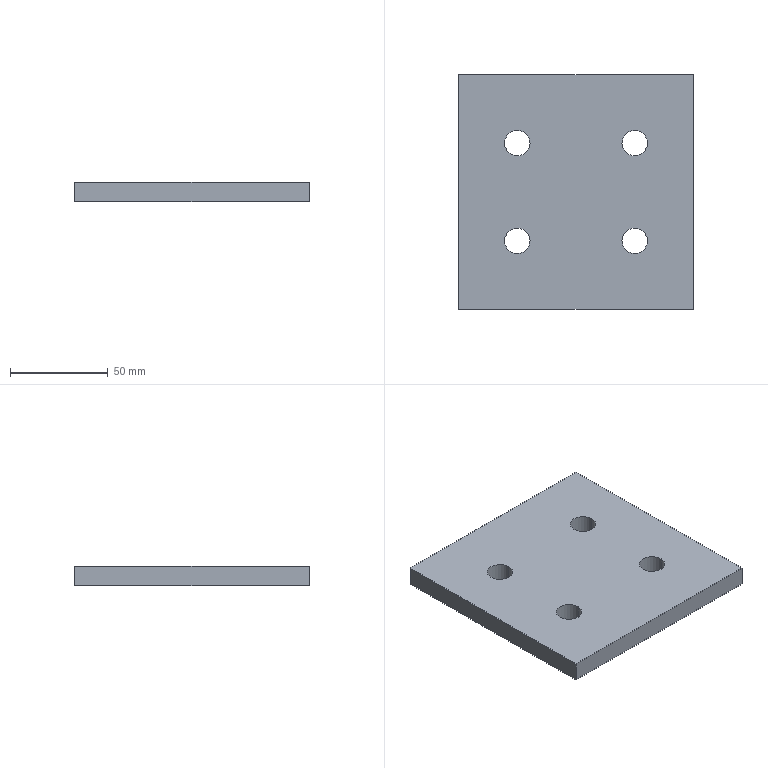Part | SolidWorks | features Extrusion 1 | 1 solid | 14 faces | box 120 x 120 x 10 mm | volume 138691 mm3 | cylinder 8 | plane 6 | commonest cylinder face diameters 13 x8
STEP:
#1=CARTESIAN_POINT('',(23.5,35.,10.));
#2=VERTEX_POINT('',#1);
#3=CARTESIAN_POINT('',(36.5,35.,10.));
#4=VERTEX_POINT('',#3);
#5=CARTESIAN_POINT('',(30.,35.,10.));
#6=DIRECTION('',(0.,0.,1.));
#7=DIRECTION('',(1.,0.,0.));
#8=AXIS2_PLACEMENT_3D('',#5,#6,#7);
#9=CIRCLE('',#8,6.5);
#10=EDGE_CURVE('',#2,#4,#9,.T.);
#11=ORIENTED_EDGE('',*,*,#10,.T.);
#12=CARTESIAN_POINT('',(36.5,35.,0.));
#13=VERTEX_POINT('',#12);
#14=CARTESIAN_POINT('',(36.5,35.,10.));
#15=DIRECTION('',(0.,0.,-1.));
#16=VECTOR('',#15,1000.);
#17=LINE('',#14,#16);
#18=EDGE_CURVE('',#4,#13,#17,.T.);
#19=ORIENTED_EDGE('',*,*,#18,.T.);
#20=CARTESIAN_POINT('',(23.5,35.,0.));
#21=VERTEX_POINT('',#20);
#22=CARTESIAN_POINT('',(30.,35.,0.));
#23=DIRECTION('',(0.,0.,1.));
#24=DIRECTION('',(1.,0.,0.));
#25=AXIS2_PLACEMENT_3D('',#22,#23,#24);
#26=CIRCLE('',#25,6.5);
#27=EDGE_CURVE('',#21,#13,#26,.T.);
#28=ORIENTED_EDGE('',*,*,#27,.F.);
#29=CARTESIAN_POINT('',(23.5,35.,10.));
#30=DIRECTION('',(0.,0.,-1.));
#31=VECTOR('',#30,1000.);
#32=LINE('',#29,#31);
#33=EDGE_CURVE('',#2,#21,#32,.T.);
#34=ORIENTED_EDGE('',*,*,#33,.F.);
#35=EDGE_LOOP('',(#11,#19,#28,#34));
#36=FACE_OUTER_BOUND('',#35,.T.);
#37=CARTESIAN_POINT('',(30.,35.,10.));
#38=DIRECTION('',(0.,0.,-1.));
#39=DIRECTION('',(-1.,0.,0.));
#40=AXIS2_PLACEMENT_3D('',#37,#38,#39);
#41=CYLINDRICAL_SURFACE('',#40,6.5);
#42=ADVANCED_FACE('',(#36),#41,.F.);
#43=CARTESIAN_POINT('',(23.5,85.,10.));
#44=VERTEX_POINT('',#43);
#45=CARTESIAN_POINT('',(36.5,85.,10.));
#46=VERTEX_POINT('',#45);
#47=CARTESIAN_POINT('',(30.,85.,10.));
#48=DIRECTION('',(0.,0.,1.));
#49=DIRECTION('',(1.,0.,0.));
#50=AXIS2_PLACEMENT_3D('',#47,#48,#49);
#51=CIRCLE('',#50,6.5);
#52=EDGE_CURVE('',#44,#46,#51,.T.);
#53=ORIENTED_EDGE('',*,*,#52,.T.);
#54=CARTESIAN_POINT('',(36.5,85.,0.));
#55=VERTEX_POINT('',#54);
#56=CARTESIAN_POINT('',(36.5,85.,10.));
#57=DIRECTION('',(0.,0.,-1.));
#58=VECTOR('',#57,1000.);
#59=LINE('',#56,#58);
#60=EDGE_CURVE('',#46,#55,#59,.T.);
#61=ORIENTED_EDGE('',*,*,#60,.T.);
#62=CARTESIAN_POINT('',(23.5,85.,0.));
#63=VERTEX_POINT('',#62);
#64=CARTESIAN_POINT('',(30.,85.,0.));
#65=DIRECTION('',(0.,0.,1.));
#66=DIRECTION('',(1.,0.,0.));
#67=AXIS2_PLACEMENT_3D('',#64,#65,#66);
#68=CIRCLE('',#67,6.5);
#69=EDGE_CURVE('',#63,#55,#68,.T.);
#70=ORIENTED_EDGE('',*,*,#69,.F.);
#71=CARTESIAN_POINT('',(23.5,85.,10.));
#72=DIRECTION('',(0.,0.,-1.));
#73=VECTOR('',#72,1000.);
#74=LINE('',#71,#73);
#75=EDGE_CURVE('',#44,#63,#74,.T.);
#76=ORIENTED_EDGE('',*,*,#75,.F.);
#77=EDGE_LOOP('',(#53,#61,#70,#76));
#78=FACE_OUTER_BOUND('',#77,.T.);
#79=CARTESIAN_POINT('',(30.,85.,10.));
#80=DIRECTION('',(0.,0.,-1.));
#81=DIRECTION('',(-1.,0.,0.));
#82=AXIS2_PLACEMENT_3D('',#79,#80,#81);
#83=CYLINDRICAL_SURFACE('',#82,6.5);
#84=ADVANCED_FACE('',(#78),#83,.F.);
#85=CARTESIAN_POINT('',(83.5,85.,10.));
#86=VERTEX_POINT('',#85);
#87=CARTESIAN_POINT('',(96.5,85.,10.));
#88=VERTEX_POINT('',#87);
#89=CARTESIAN_POINT('',(90.,85.,10.));
#90=DIRECTION('',(0.,0.,1.));
#91=DIRECTION('',(1.,0.,0.));
#92=AXIS2_PLACEMENT_3D('',#89,#90,#91);
#93=CIRCLE('',#92,6.5);
#94=EDGE_CURVE('',#86,#88,#93,.T.);
#95=ORIENTED_EDGE('',*,*,#94,.T.);
#96=CARTESIAN_POINT('',(96.5,85.,0.));
#97=VERTEX_POINT('',#96);
#98=CARTESIAN_POINT('',(96.5,85.,10.));
#99=DIRECTION('',(0.,0.,-1.));
#100=VECTOR('',#99,1000.);
#101=LINE('',#98,#100);
#102=EDGE_CURVE('',#88,#97,#101,.T.);
#103=ORIENTED_EDGE('',*,*,#102,.T.);
#104=CARTESIAN_POINT('',(83.5,85.,0.));
#105=VERTEX_POINT('',#104);
#106=CARTESIAN_POINT('',(90.,85.,0.));
#107=DIRECTION('',(0.,0.,1.));
#108=DIRECTION('',(1.,0.,0.));
#109=AXIS2_PLACEMENT_3D('',#106,#107,#108);
#110=CIRCLE('',#109,6.5);
#111=EDGE_CURVE('',#105,#97,#110,.T.);
#112=ORIENTED_EDGE('',*,*,#111,.F.);
#113=CARTESIAN_POINT('',(83.5,85.,10.));
#114=DIRECTION('',(0.,0.,-1.));
#115=VECTOR('',#114,1000.);
#116=LINE('',#113,#115);
#117=EDGE_CURVE('',#86,#105,#116,.T.);
#118=ORIENTED_EDGE('',*,*,#117,.F.);
#119=EDGE_LOOP('',(#95,#103,#112,#118));
#120=FACE_OUTER_BOUND('',#119,.T.);
#121=CARTESIAN_POINT('',(90.,85.,10.));
#122=DIRECTION('',(0.,0.,-1.));
#123=DIRECTION('',(-1.,0.,0.));
#124=AXIS2_PLACEMENT_3D('',#121,#122,#123);
#125=CYLINDRICAL_SURFACE('',#124,6.5);
#126=ADVANCED_FACE('',(#120),#125,.F.);
#127=CARTESIAN_POINT('',(83.5,35.,10.));
#128=VERTEX_POINT('',#127);
#129=CARTESIAN_POINT('',(96.5,35.,10.));
#130=VERTEX_POINT('',#129);
#131=CARTESIAN_POINT('',(90.,35.,10.));
#132=DIRECTION('',(0.,0.,1.));
#133=DIRECTION('',(1.,0.,0.));
#134=AXIS2_PLACEMENT_3D('',#131,#132,#133);
#135=CIRCLE('',#134,6.5);
#136=EDGE_CURVE('',#128,#130,#135,.T.);
#137=ORIENTED_EDGE('',*,*,#136,.T.);
#138=CARTESIAN_POINT('',(96.5,35.,0.));
#139=VERTEX_POINT('',#138);
#140=CARTESIAN_POINT('',(96.5,35.,10.));
#141=DIRECTION('',(0.,0.,-1.));
#142=VECTOR('',#141,1000.);
#143=LINE('',#140,#142);
#144=EDGE_CURVE('',#130,#139,#143,.T.);
#145=ORIENTED_EDGE('',*,*,#144,.T.);
#146=CARTESIAN_POINT('',(83.5,35.,0.));
#147=VERTEX_POINT('',#146);
#148=CARTESIAN_POINT('',(90.,35.,0.));
#149=DIRECTION('',(0.,0.,1.));
#150=DIRECTION('',(1.,0.,0.));
#151=AXIS2_PLACEMENT_3D('',#148,#149,#150);
#152=CIRCLE('',#151,6.5);
#153=EDGE_CURVE('',#147,#139,#152,.T.);
#154=ORIENTED_EDGE('',*,*,#153,.F.);
#155=CARTESIAN_POINT('',(83.5,35.,10.));
#156=DIRECTION('',(0.,0.,-1.));
#157=VECTOR('',#156,1000.);
#158=LINE('',#155,#157);
#159=EDGE_CURVE('',#128,#147,#158,.T.);
#160=ORIENTED_EDGE('',*,*,#159,.F.);
#161=EDGE_LOOP('',(#137,#145,#154,#160));
#162=FACE_OUTER_BOUND('',#161,.T.);
#163=CARTESIAN_POINT('',(90.,35.,10.));
#164=DIRECTION('',(0.,0.,-1.));
#165=DIRECTION('',(-1.,0.,0.));
#166=AXIS2_PLACEMENT_3D('',#163,#164,#165);
#167=CYLINDRICAL_SURFACE('',#166,6.5);
#168=ADVANCED_FACE('',(#162),#167,.F.);
#169=CARTESIAN_POINT('',(120.,0.,0.));
#170=VERTEX_POINT('',#169);
#171=CARTESIAN_POINT('',(0.,0.,0.));
#172=VERTEX_POINT('',#171);
#173=CARTESIAN_POINT('',(0.,0.,0.));
#174=DIRECTION('',(-1.,0.,0.));
#175=VECTOR('',#174,1000.);
#176=LINE('',#173,#175);
#177=EDGE_CURVE('',#170,#172,#176,.T.);
#178=ORIENTED_EDGE('',*,*,#177,.F.);
#179=CARTESIAN_POINT('',(120.,0.,10.));
#180=VERTEX_POINT('',#179);
#181=CARTESIAN_POINT('',(120.,0.,10.));
#182=DIRECTION('',(0.,0.,-1.));
#183=VECTOR('',#182,1000.);
#184=LINE('',#181,#183);
#185=EDGE_CURVE('',#180,#170,#184,.T.);
#186=ORIENTED_EDGE('',*,*,#185,.F.);
#187=CARTESIAN_POINT('',(0.,0.,10.));
#188=VERTEX_POINT('',#187);
#189=CARTESIAN_POINT('',(0.,0.,10.));
#190=DIRECTION('',(-1.,0.,0.));
#191=VECTOR('',#190,1000.);
#192=LINE('',#189,#191);
#193=EDGE_CURVE('',#180,#188,#192,.T.);
#194=ORIENTED_EDGE('',*,*,#193,.T.);
#195=CARTESIAN_POINT('',(0.,0.,10.));
#196=DIRECTION('',(0.,0.,-1.));
#197=VECTOR('',#196,1000.);
#198=LINE('',#195,#197);
#199=EDGE_CURVE('',#188,#172,#198,.T.);
#200=ORIENTED_EDGE('',*,*,#199,.T.);
#201=EDGE_LOOP('',(#178,#186,#194,#200));
#202=FACE_OUTER_BOUND('',#201,.T.);
#203=CARTESIAN_POINT('',(0.,0.,10.));
#204=DIRECTION('',(0.,-1.,0.));
#205=DIRECTION('',(0.,0.,-1.));
#206=AXIS2_PLACEMENT_3D('',#203,#204,#205);
#207=PLANE('',#206);
#208=ADVANCED_FACE('',(#202),#207,.T.);
#209=CARTESIAN_POINT('',(120.,120.,0.));
#210=VERTEX_POINT('',#209);
#211=CARTESIAN_POINT('',(120.,0.,0.));
#212=DIRECTION('',(0.,-1.,0.));
#213=VECTOR('',#212,1000.);
#214=LINE('',#211,#213);
#215=EDGE_CURVE('',#210,#170,#214,.T.);
#216=ORIENTED_EDGE('',*,*,#215,.F.);
#217=CARTESIAN_POINT('',(120.,120.,10.));
#218=VERTEX_POINT('',#217);
#219=CARTESIAN_POINT('',(120.,120.,10.));
#220=DIRECTION('',(0.,0.,-1.));
#221=VECTOR('',#220,1000.);
#222=LINE('',#219,#221);
#223=EDGE_CURVE('',#218,#210,#222,.T.);
#224=ORIENTED_EDGE('',*,*,#223,.F.);
#225=CARTESIAN_POINT('',(120.,0.,10.));
#226=DIRECTION('',(0.,-1.,0.));
#227=VECTOR('',#226,1000.);
#228=LINE('',#225,#227);
#229=EDGE_CURVE('',#218,#180,#228,.T.);
#230=ORIENTED_EDGE('',*,*,#229,.T.);
#231=ORIENTED_EDGE('',*,*,#185,.T.);
#232=EDGE_LOOP('',(#216,#224,#230,#231));
#233=FACE_OUTER_BOUND('',#232,.T.);
#234=CARTESIAN_POINT('',(120.,0.,10.));
#235=DIRECTION('',(1.,0.,0.));
#236=DIRECTION('',(0.,1.,0.));
#237=AXIS2_PLACEMENT_3D('',#234,#235,#236);
#238=PLANE('',#237);
#239=ADVANCED_FACE('',(#233),#238,.T.);
#240=CARTESIAN_POINT('',(0.,120.,0.));
#241=VERTEX_POINT('',#240);
#242=CARTESIAN_POINT('',(0.,120.,0.));
#243=DIRECTION('',(1.,0.,0.));
#244=VECTOR('',#243,1000.);
#245=LINE('',#242,#244);
#246=EDGE_CURVE('',#241,#210,#245,.T.);
#247=ORIENTED_EDGE('',*,*,#246,.F.);
#248=CARTESIAN_POINT('',(0.,120.,10.));
#249=VERTEX_POINT('',#248);
#250=CARTESIAN_POINT('',(0.,120.,10.));
#251=DIRECTION('',(0.,0.,-1.));
#252=VECTOR('',#251,1000.);
#253=LINE('',#250,#252);
#254=EDGE_CURVE('',#249,#241,#253,.T.);
#255=ORIENTED_EDGE('',*,*,#254,.F.);
#256=CARTESIAN_POINT('',(0.,120.,10.));
#257=DIRECTION('',(1.,0.,0.));
#258=VECTOR('',#257,1000.);
#259=LINE('',#256,#258);
#260=EDGE_CURVE('',#249,#218,#259,.T.);
#261=ORIENTED_EDGE('',*,*,#260,.T.);
#262=ORIENTED_EDGE('',*,*,#223,.T.);
#263=EDGE_LOOP('',(#247,#255,#261,#262));
#264=FACE_OUTER_BOUND('',#263,.T.);
#265=CARTESIAN_POINT('',(0.,120.,10.));
#266=DIRECTION('',(0.,1.,0.));
#267=DIRECTION('',(0.,0.,1.));
#268=AXIS2_PLACEMENT_3D('',#265,#266,#267);
#269=PLANE('',#268);
#270=ADVANCED_FACE('',(#264),#269,.T.);
#271=CARTESIAN_POINT('',(0.,0.,0.));
#272=DIRECTION('',(0.,1.,0.));
#273=VECTOR('',#272,1000.);
#274=LINE('',#271,#273);
#275=EDGE_CURVE('',#172,#241,#274,.T.);
#276=ORIENTED_EDGE('',*,*,#275,.F.);
#277=ORIENTED_EDGE('',*,*,#199,.F.);
#278=CARTESIAN_POINT('',(0.,0.,10.));
#279=DIRECTION('',(0.,1.,0.));
#280=VECTOR('',#279,1000.);
#281=LINE('',#278,#280);
#282=EDGE_CURVE('',#188,#249,#281,.T.);
#283=ORIENTED_EDGE('',*,*,#282,.T.);
#284=ORIENTED_EDGE('',*,*,#254,.T.);
#285=EDGE_LOOP('',(#276,#277,#283,#284));
#286=FACE_OUTER_BOUND('',#285,.T.);
#287=CARTESIAN_POINT('',(0.,0.,10.));
#288=DIRECTION('',(-1.,0.,0.));
#289=DIRECTION('',(0.,0.,1.));
#290=AXIS2_PLACEMENT_3D('',#287,#288,#289);
#291=PLANE('',#290);
#292=ADVANCED_FACE('',(#286),#291,.T.);
#293=ORIENTED_EDGE('',*,*,#144,.F.);
#294=CARTESIAN_POINT('',(90.,35.,10.));
#295=DIRECTION('',(0.,0.,1.));
#296=DIRECTION('',(1.,0.,0.));
#297=AXIS2_PLACEMENT_3D('',#294,#295,#296);
#298=CIRCLE('',#297,6.5);
#299=EDGE_CURVE('',#130,#128,#298,.T.);
#300=ORIENTED_EDGE('',*,*,#299,.T.);
#301=ORIENTED_EDGE('',*,*,#159,.T.);
#302=CARTESIAN_POINT('',(90.,35.,0.));
#303=DIRECTION('',(0.,0.,1.));
#304=DIRECTION('',(1.,0.,0.));
#305=AXIS2_PLACEMENT_3D('',#302,#303,#304);
#306=CIRCLE('',#305,6.5);
#307=EDGE_CURVE('',#139,#147,#306,.T.);
#308=ORIENTED_EDGE('',*,*,#307,.F.);
#309=EDGE_LOOP('',(#293,#300,#301,#308));
#310=FACE_OUTER_BOUND('',#309,.T.);
#311=CARTESIAN_POINT('',(90.,35.,10.));
#312=DIRECTION('',(0.,0.,-1.));
#313=DIRECTION('',(-1.,0.,0.));
#314=AXIS2_PLACEMENT_3D('',#311,#312,#313);
#315=CYLINDRICAL_SURFACE('',#314,6.5);
#316=ADVANCED_FACE('',(#310),#315,.F.);
#317=ORIENTED_EDGE('',*,*,#102,.F.);
#318=CARTESIAN_POINT('',(90.,85.,10.));
#319=DIRECTION('',(0.,0.,1.));
#320=DIRECTION('',(1.,0.,0.));
#321=AXIS2_PLACEMENT_3D('',#318,#319,#320);
#322=CIRCLE('',#321,6.5);
#323=EDGE_CURVE('',#88,#86,#322,.T.);
#324=ORIENTED_EDGE('',*,*,#323,.T.);
#325=ORIENTED_EDGE('',*,*,#117,.T.);
#326=CARTESIAN_POINT('',(90.,85.,0.));
#327=DIRECTION('',(0.,0.,1.));
#328=DIRECTION('',(1.,0.,0.));
#329=AXIS2_PLACEMENT_3D('',#326,#327,#328);
#330=CIRCLE('',#329,6.5);
#331=EDGE_CURVE('',#97,#105,#330,.T.);
#332=ORIENTED_EDGE('',*,*,#331,.F.);
#333=EDGE_LOOP('',(#317,#324,#325,#332));
#334=FACE_OUTER_BOUND('',#333,.T.);
#335=CARTESIAN_POINT('',(90.,85.,10.));
#336=DIRECTION('',(0.,0.,-1.));
#337=DIRECTION('',(-1.,0.,0.));
#338=AXIS2_PLACEMENT_3D('',#335,#336,#337);
#339=CYLINDRICAL_SURFACE('',#338,6.5);
#340=ADVANCED_FACE('',(#334),#339,.F.);
#341=ORIENTED_EDGE('',*,*,#60,.F.);
#342=CARTESIAN_POINT('',(30.,85.,10.));
#343=DIRECTION('',(0.,0.,1.));
#344=DIRECTION('',(1.,0.,0.));
#345=AXIS2_PLACEMENT_3D('',#342,#343,#344);
#346=CIRCLE('',#345,6.5);
#347=EDGE_CURVE('',#46,#44,#346,.T.);
#348=ORIENTED_EDGE('',*,*,#347,.T.);
#349=ORIENTED_EDGE('',*,*,#75,.T.);
#350=CARTESIAN_POINT('',(30.,85.,0.));
#351=DIRECTION('',(0.,0.,1.));
#352=DIRECTION('',(1.,0.,0.));
#353=AXIS2_PLACEMENT_3D('',#350,#351,#352);
#354=CIRCLE('',#353,6.5);
#355=EDGE_CURVE('',#55,#63,#354,.T.);
#356=ORIENTED_EDGE('',*,*,#355,.F.);
#357=EDGE_LOOP('',(#341,#348,#349,#356));
#358=FACE_OUTER_BOUND('',#357,.T.);
#359=CARTESIAN_POINT('',(30.,85.,10.));
#360=DIRECTION('',(0.,0.,-1.));
#361=DIRECTION('',(-1.,0.,0.));
#362=AXIS2_PLACEMENT_3D('',#359,#360,#361);
#363=CYLINDRICAL_SURFACE('',#362,6.5);
#364=ADVANCED_FACE('',(#358),#363,.F.);
#365=ORIENTED_EDGE('',*,*,#18,.F.);
#366=CARTESIAN_POINT('',(30.,35.,10.));
#367=DIRECTION('',(0.,0.,1.));
#368=DIRECTION('',(1.,0.,0.));
#369=AXIS2_PLACEMENT_3D('',#366,#367,#368);
#370=CIRCLE('',#369,6.5);
#371=EDGE_CURVE('',#4,#2,#370,.T.);
#372=ORIENTED_EDGE('',*,*,#371,.T.);
#373=ORIENTED_EDGE('',*,*,#33,.T.);
#374=CARTESIAN_POINT('',(30.,35.,0.));
#375=DIRECTION('',(0.,0.,1.));
#376=DIRECTION('',(1.,0.,0.));
#377=AXIS2_PLACEMENT_3D('',#374,#375,#376);
#378=CIRCLE('',#377,6.5);
#379=EDGE_CURVE('',#13,#21,#378,.T.);
#380=ORIENTED_EDGE('',*,*,#379,.F.);
#381=EDGE_LOOP('',(#365,#372,#373,#380));
#382=FACE_OUTER_BOUND('',#381,.T.);
#383=CARTESIAN_POINT('',(30.,35.,10.));
#384=DIRECTION('',(0.,0.,-1.));
#385=DIRECTION('',(-1.,0.,0.));
#386=AXIS2_PLACEMENT_3D('',#383,#384,#385);
#387=CYLINDRICAL_SURFACE('',#386,6.5);
#388=ADVANCED_FACE('',(#382),#387,.F.);
#389=ORIENTED_EDGE('',*,*,#52,.F.);
#390=ORIENTED_EDGE('',*,*,#347,.F.);
#391=EDGE_LOOP('',(#389,#390));
#392=FACE_BOUND('',#391,.T.);
#393=ORIENTED_EDGE('',*,*,#94,.F.);
#394=ORIENTED_EDGE('',*,*,#323,.F.);
#395=EDGE_LOOP('',(#393,#394));
#396=FACE_BOUND('',#395,.T.);
#397=ORIENTED_EDGE('',*,*,#136,.F.);
#398=ORIENTED_EDGE('',*,*,#299,.F.);
#399=EDGE_LOOP('',(#397,#398));
#400=FACE_BOUND('',#399,.T.);
#401=ORIENTED_EDGE('',*,*,#193,.F.);
#402=ORIENTED_EDGE('',*,*,#229,.F.);
#403=ORIENTED_EDGE('',*,*,#260,.F.);
#404=ORIENTED_EDGE('',*,*,#282,.F.);
#405=EDGE_LOOP('',(#401,#402,#403,#404));
#406=FACE_OUTER_BOUND('',#405,.T.);
#407=ORIENTED_EDGE('',*,*,#10,.F.);
#408=ORIENTED_EDGE('',*,*,#371,.F.);
#409=EDGE_LOOP('',(#407,#408));
#410=FACE_BOUND('',#409,.T.);
#411=CARTESIAN_POINT('',(0.,0.,10.));
#412=DIRECTION('',(0.,0.,1.));
#413=DIRECTION('',(1.,0.,0.));
#414=AXIS2_PLACEMENT_3D('',#411,#412,#413);
#415=PLANE('',#414);
#416=ADVANCED_FACE('',(#392,#396,#400,#406,#410),#415,.T.);
#417=ORIENTED_EDGE('',*,*,#69,.T.);
#418=ORIENTED_EDGE('',*,*,#355,.T.);
#419=EDGE_LOOP('',(#417,#418));
#420=FACE_BOUND('',#419,.T.);
#421=ORIENTED_EDGE('',*,*,#111,.T.);
#422=ORIENTED_EDGE('',*,*,#331,.T.);
#423=EDGE_LOOP('',(#421,#422));
#424=FACE_BOUND('',#423,.T.);
#425=ORIENTED_EDGE('',*,*,#153,.T.);
#426=ORIENTED_EDGE('',*,*,#307,.T.);
#427=EDGE_LOOP('',(#425,#426));
#428=FACE_BOUND('',#427,.T.);
#429=ORIENTED_EDGE('',*,*,#177,.T.);
#430=ORIENTED_EDGE('',*,*,#275,.T.);
#431=ORIENTED_EDGE('',*,*,#246,.T.);
#432=ORIENTED_EDGE('',*,*,#215,.T.);
#433=EDGE_LOOP('',(#429,#430,#431,#432));
#434=FACE_OUTER_BOUND('',#433,.T.);
#435=ORIENTED_EDGE('',*,*,#27,.T.);
#436=ORIENTED_EDGE('',*,*,#379,.T.);
#437=EDGE_LOOP('',(#435,#436));
#438=FACE_BOUND('',#437,.T.);
#439=CARTESIAN_POINT('',(0.,0.,0.));
#440=DIRECTION('',(0.,0.,1.));
#441=DIRECTION('',(1.,0.,0.));
#442=AXIS2_PLACEMENT_3D('',#439,#440,#441);
#443=PLANE('',#442);
#444=ADVANCED_FACE('',(#420,#424,#428,#434,#438),#443,.F.);
#445=CLOSED_SHELL('',(#42,#84,#126,#168,#208,#239,#270,#292,#316,#340,#364,#388,#416,#444));
#446=MANIFOLD_SOLID_BREP('',#445);
#447=CARTESIAN_POINT('',(0.,0.,0.));
#448=DIRECTION('',(0.,0.,1.));
#449=DIRECTION('',(1.,0.,0.));
#450=AXIS2_PLACEMENT_3D('',#447,#448,#449);
#451=(LENGTH_UNIT()NAMED_UNIT(*)SI_UNIT(.MILLI.,.METRE.));
#452=UNCERTAINTY_MEASURE_WITH_UNIT(LENGTH_MEASURE(0.00001),#451,'','');
#453=(NAMED_UNIT(*)PLANE_ANGLE_UNIT()SI_UNIT($,.RADIAN.));
#454=(NAMED_UNIT(*)SI_UNIT($,.STERADIAN.)SOLID_ANGLE_UNIT());
#455=(GEOMETRIC_REPRESENTATION_CONTEXT(3)GLOBAL_UNCERTAINTY_ASSIGNED_CONTEXT((#452))GLOBAL_UNIT_ASSIGNED_CONTEXT((#451,#453,#454))REPRESENTATION_CONTEXT('',''));
#456=ADVANCED_BREP_SHAPE_REPRESENTATION('',(#446,#450),#455);